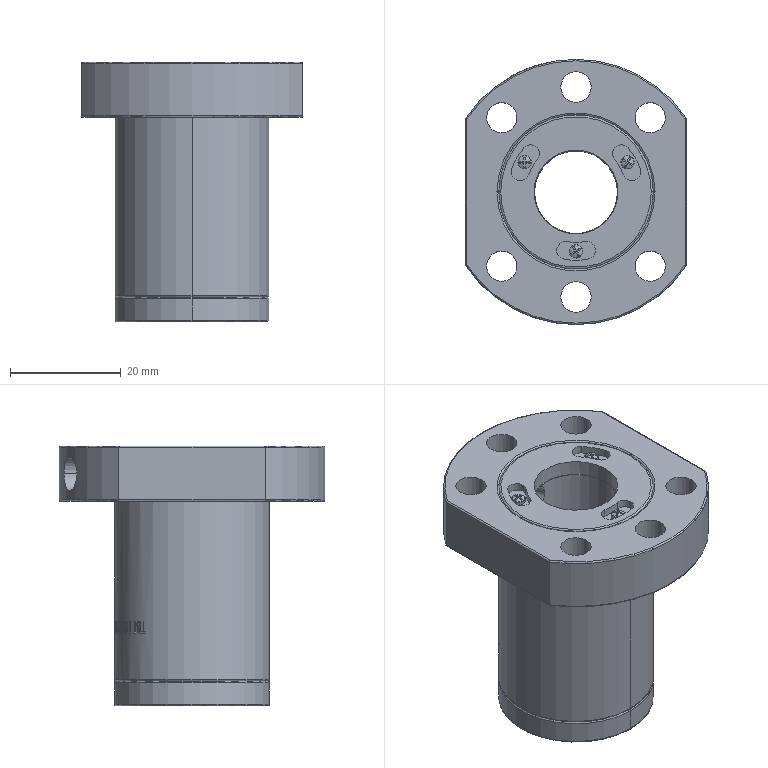Part | STEP file | 1 solid | 395 faces | box 40 x 48 x 47 mm | volume 29180 mm3 | plane 132 | spline 120 | cylinder 105 | torus 26 | sphere 12 | commonest cylinder face diameters 3.25 x18 28 x18 28.02 x17 2.438 x12 5.5 x12 18.25 x6